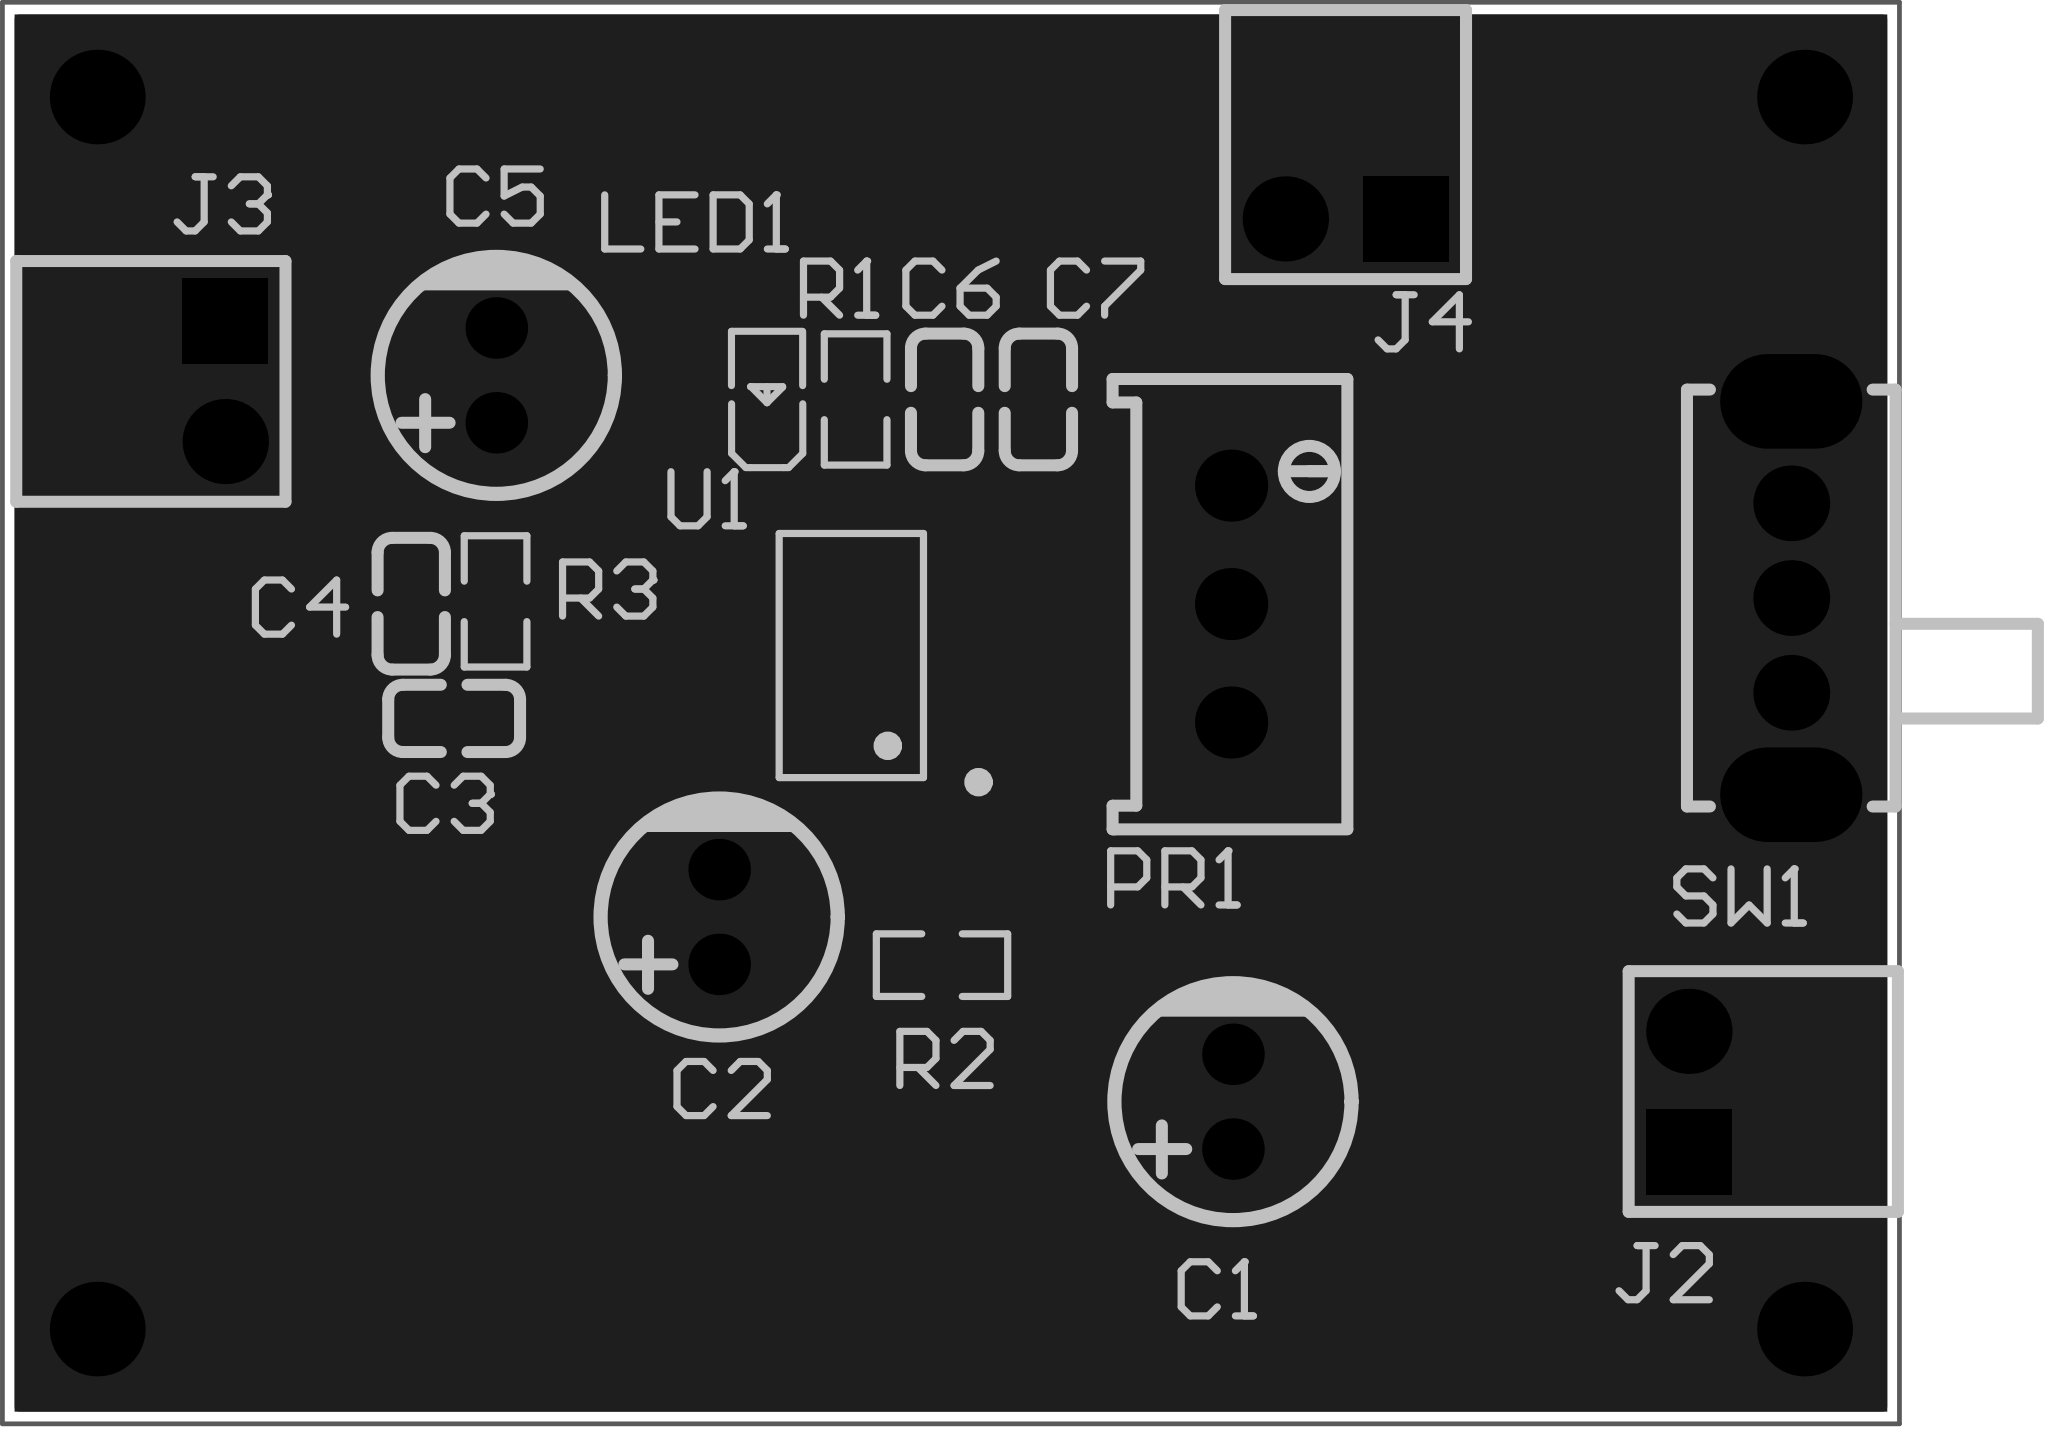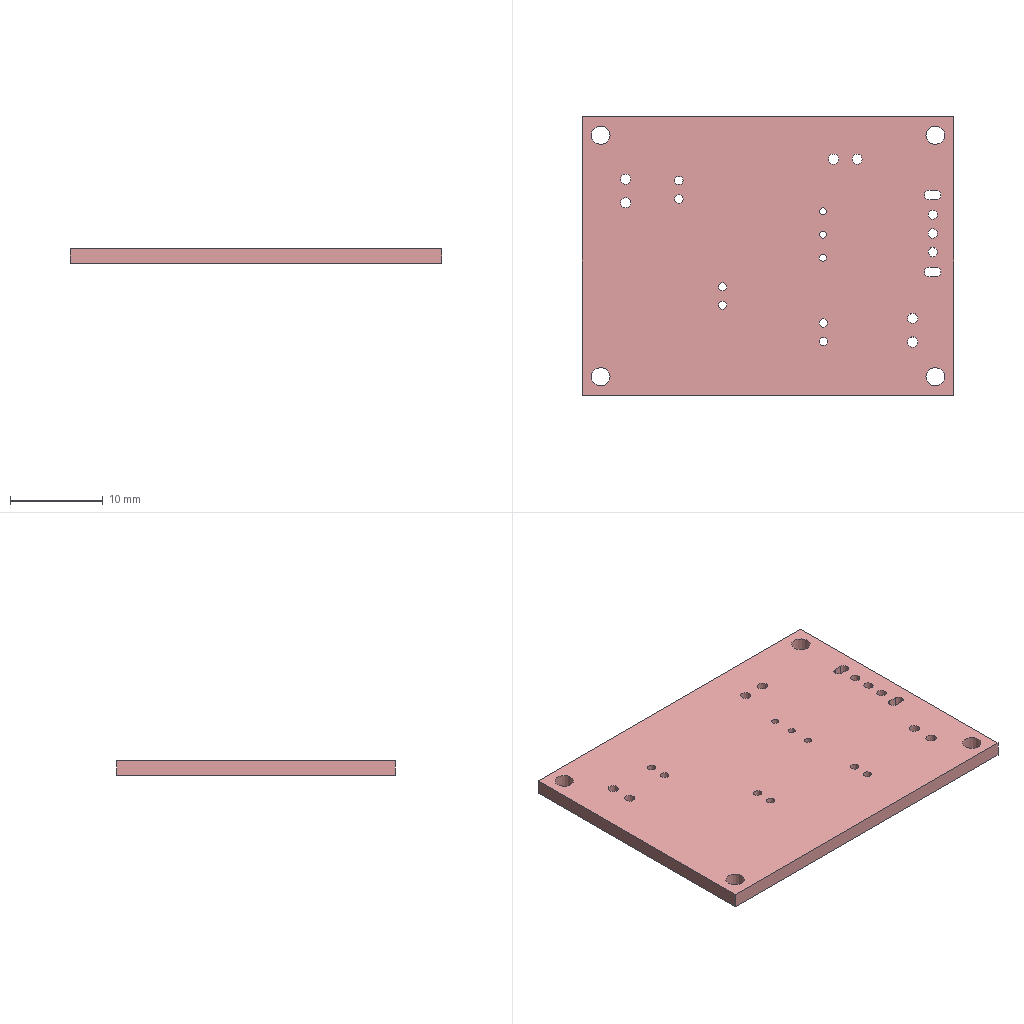Circuit board layout | Altium Designer | box 40 x 30 x 1.6 mm
Layer stack:
# Altium Designer layer stack of  (unit mm; dielectric type: 0 none, 1 core, 2 prepreg, 3 surface material)
index,name,kind,layer,copper_thickness_mm,dielectric_type,dielectric_thickness_mm,dielectric_material,dielectric_constant
0,Top Paste Mask Layer,other,,,,,,
1,Top Silkscreen Layer,other,,,,,,
2,Top Solder Mask Layer,dielectric,,,3,0.01,,3.3
3,Top Layer,copper,Top Layer,0.035,,,,
4,Dielectric1,dielectric,,,3,1.51,FR4,4.5
5,Bottom Layer,copper,Bottom Layer,0.035,,,,
6,Bottom Solder Mask Layer,dielectric,,,3,0.01,,3.3
7,Bottom Silkscreen Layer,other,,,,,,
8,Bottom Paste Mask Layer,other,,,,,,
# drill layer pairs: low layer,high layer
drill_pair,Top Layer,Bottom Layer
Part placement:
Designator,Comment,Layer,Footprint,Center-X(mm),Center-Y(mm),Rotation
C1,2.2uF,TopLayer,CAP-TH_BD5.0-P2.00-D0.8-FD-10UF50VC110GL,102.147,82.999,90
J2,,TopLayer,HDR-TH_2P-P2.54-V-M-1,111.76,83.213,90
C4,0.22uF,TopLayer,C0603,84.821,93.507,270
C3,100nF,TopLayer,C0603,85.725,91.087,0
C6,0.1uF,TopLayer,C0603,96.067,97.818,270
C7,220uF,TopLayer,C0603,98.044,97.818,270
SW1,,TopLayer,拨动开关_侧,113.919,93.627,90
C5,470uF,TopLayer,CAP-TH_BD5.0-P2.00-D0.8-FD-10UF50VC110GL,86.614,98.326,90
J3,,TopLayer,HDR-TH_2P-P2.54-V-M-1,80.899,98.199,270
J4,,TopLayer,HDR-TH_2P-P2.54-V-M-1,104.521,101.628,180
LED1,,TopLayer,LED_0603,92.329,97.868,90
U1,LM386DTR(XBLW),TopLayer,SOP-8_L4.9-W3.9-P1.27-LS6.0-BL,94.1,92.414,90
R1,1K,TopLayer,R0603,94.191,97.818,270
PR1,10kO,TopLayer,R_3296,102.108,93.5,270
R3,22E,TopLayer,R0603,86.599,93.557,90
C2,10uF,TopLayer,CAP-TH_BD5.0-P2.00-D0.8-FD-10UF50VC110GL,91.313,86.896,90
R2,2K2,TopLayer,R0603,96.012,85.88,0
Pad and via stacks:
# Altium Designer via and pad stacks of  (unit mm). Each distinct definition once, with the count of objects using it.
# via: kind,start_layer,end_layer,hole_mm,diameter_mm,mode(0 simple;1 top-mid-bottom;2 full stack),diameter_per_layer,count,example_net
# pad: kind,layer,hole_mm,hole_type(0 round;1 square;2 slot),plating,top_size,top_shape(1 round;2 rect;3 octagon;9 rounded rect),mid_size,bottom_size,mode,footprint,size_per_layer,count,example
pad,Multi-Layer,0.9,0,plated,1.3x1.3,1,1.3x1.3,1.3x1.3,0,CAP-TH_BD5.0-P2.00-D0.8-FD-10UF50VC110GL,,6,C1.2
pad,Multi-Layer,1.1,0,plated,1.8x1.8,1,1.8x1.8,1.8x1.8,0,HDR-TH_2P-P2.54-V-M-1,,3,J2.2
pad,Multi-Layer,1.1,0,plated,1.8x1.8,2,1.8x1.8,1.8x1.8,0,HDR-TH_2P-P2.54-V-M-1,,3,J2.1
pad,Multi-Layer,2,0,plated,2x2,1,2x2,2x2,0,,,4,1
pad,Multi-Layer,1.001,0,plated,1.6x1.6,1,1.6x1.6,1.6x1.6,0,\u00B2\u00A6\u00B6\u00AF\u00BF\u00AA\u00B9\u00D8_\u00B2\u00E0,,3,SW1.1
pad,Multi-Layer,1.001,2,plated,3x1.999,1,3x1.999,3x1.999,0,\u00B2\u00A6\u00B6\u00AF\u00BF\u00AA\u00B9\u00D8_\u00B2\u00E0,,2,SW1.4
pad,Multi-Layer,0.762,0,plated,1.524x1.524,1,1.524x1.524,1.524x1.524,0,R_3296,,3,PR1.2
pad,Top Layer,0,0,plated,0.8x0.9,2,0.8x0.9,0.8x0.9,0,C0603,,8,C4.2
pad,Top Layer,0,0,plated,0.8001x0.8001,2,0.8001x0.8001,0.8001x0.8001,0,LED_0603,,2,LED1.1
pad,Top Layer,0,0,plated,0.63x1.865,1,0.63x1.865,0.63x1.865,0,SOP-8_L4.9-W3.9-P1.27-LS6.0-BL,,8,U1.1
pad,Top Layer,0,0,plated,0.8065x0.864,2,0.8065x0.864,0.8065x0.864,0,R0603,,6,R1.2
Copper pours:
name,layer,net,type(0 solid;1 hatched;2 none)
Top Layer-GND,Top Layer,GND,0
Bottom Layer-GND,Bottom Layer,GND,0
Design rules, without the lines most boards share:
# Altium Designer design rules of  (exported by Altium Designer, unit mm)
# columns: name | kind | enabled | priority | scope1 | scope2 | descriptor | typed fields (field=value)
creepage | 65 | enabled | 1 | All | All | Creepage Distance Constraint =(0mil) (All),(All) |